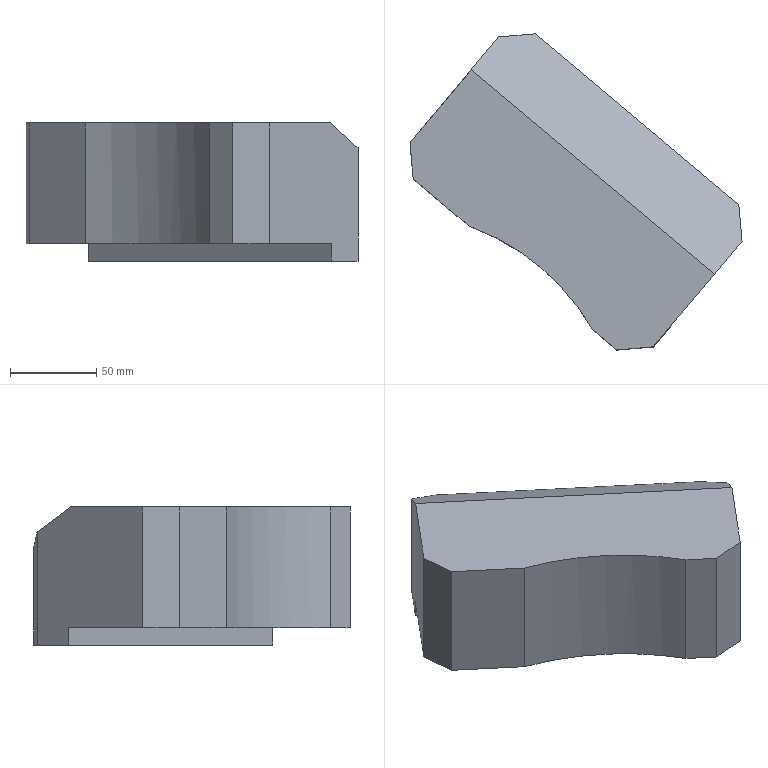Part | NX | features solid 2 | 1 solid | 31 faces | box 192.375 x 183.254 x 80 mm | volume 1311532 mm3 | plane 14 | cylinder 8 | cone 8 | spline 1 | commonest cylinder face diameters 10 x4 12 x4
STEP:
#1=CARTESIAN_POINT('',(626.964,495.071,0.000000024));
#2=VERTEX_POINT('',#1);
#3=CARTESIAN_POINT('',(621.964,495.071,0.000000024));
#4=DIRECTION('',(0.,0.,1.));
#5=DIRECTION('',(1.,0.,0.));
#6=AXIS2_PLACEMENT_3D('',#3,#4,#5);
#7=CIRCLE('',#6,5.);
#8=EDGE_CURVE('',#2,#2,#7,.T.);
#9=ORIENTED_EDGE('',*,*,#8,.T.);
#10=EDGE_LOOP('',(#9));
#11=FACE_BOUND('',#10,.T.);
#12=CARTESIAN_POINT('',(603.499,560.45,0.000000024));
#13=VERTEX_POINT('',#12);
#14=CARTESIAN_POINT('',(598.499,560.45,0.000000024));
#15=DIRECTION('',(0.,0.,1.));
#16=DIRECTION('',(1.,0.,0.));
#17=AXIS2_PLACEMENT_3D('',#14,#15,#16);
#18=CIRCLE('',#17,5.);
#19=EDGE_CURVE('',#13,#13,#18,.T.);
#20=ORIENTED_EDGE('',*,*,#19,.T.);
#21=EDGE_LOOP('',(#20));
#22=FACE_BOUND('',#21,.T.);
#23=CARTESIAN_POINT('',(650.461,521.883,0.000000024));
#24=VERTEX_POINT('',#23);
#25=CARTESIAN_POINT('',(644.461,521.883,0.000000024));
#26=DIRECTION('',(0.,0.,1.));
#27=DIRECTION('',(1.,0.,0.));
#28=AXIS2_PLACEMENT_3D('',#25,#26,#27);
#29=CIRCLE('',#28,6.);
#30=EDGE_CURVE('',#24,#24,#29,.T.);
#31=ORIENTED_EDGE('',*,*,#30,.T.);
#32=EDGE_LOOP('',(#31));
#33=FACE_BOUND('',#32,.T.);
#34=CARTESIAN_POINT('',(623.65,544.38,0.000000024));
#35=VERTEX_POINT('',#34);
#36=CARTESIAN_POINT('',(617.65,544.38,0.000000024));
#37=DIRECTION('',(0.,0.,1.));
#38=DIRECTION('',(1.,0.,0.));
#39=AXIS2_PLACEMENT_3D('',#36,#37,#38);
#40=CIRCLE('',#39,6.);
#41=EDGE_CURVE('',#35,#35,#40,.T.);
#42=ORIENTED_EDGE('',*,*,#41,.T.);
#43=EDGE_LOOP('',(#42));
#44=FACE_BOUND('',#43,.T.);
#45=CARTESIAN_POINT('',(523.703,550.108,0.000000024));
#46=VERTEX_POINT('',#45);
#47=CARTESIAN_POINT('',(595.572,489.803,0.000000024));
#48=VERTEX_POINT('',#47);
#49=CARTESIAN_POINT('',(523.703,550.108,0.000000024));
#50=CARTESIAN_POINT('',(531.205,547.402,0.000000024));
#51=CARTESIAN_POINT('',(545.792,540.631,0.000000024));
#52=CARTESIAN_POINT('',(565.448,526.903,0.000000024));
#53=CARTESIAN_POINT('',(582.431,509.864,0.000000024));
#54=CARTESIAN_POINT('',(591.599,496.685,0.000000024));
#55=CARTESIAN_POINT('',(595.572,489.803,0.000000024));
#56=B_SPLINE_CURVE_WITH_KNOTS('',3,(#49,#50,#51,#52,#53,#54,#55),.UNSPECIFIED.,.F.,.F.,(4,1,1,1,4),(0.2128,0.2368,0.2608,0.2847,0.3087),.UNSPECIFIED.);
#57=EDGE_CURVE('',#46,#48,#56,.T.);
#58=ORIENTED_EDGE('',*,*,#57,.F.);
#59=CARTESIAN_POINT('',(491.261,577.331,0.000000024));
#60=VERTEX_POINT('',#59);
#61=CARTESIAN_POINT('',(467.513,597.257,0.000000024));
#62=DIRECTION('',(0.766,-0.6428,0.));
#63=VECTOR('',#62,1000.);
#64=LINE('',#61,#63);
#65=EDGE_CURVE('',#60,#46,#64,.T.);
#66=ORIENTED_EDGE('',*,*,#65,.F.);
#67=CARTESIAN_POINT('',(489.412,598.463,0.000000024));
#68=VERTEX_POINT('',#67);
#69=CARTESIAN_POINT('',(491.261,577.331,0.000000024));
#70=DIRECTION('',(0.08716,-0.9962,0.));
#71=VECTOR('',#70,1000.);
#72=LINE('',#69,#71);
#73=EDGE_CURVE('',#68,#60,#72,.T.);
#74=ORIENTED_EDGE('',*,*,#73,.F.);
#75=CARTESIAN_POINT('',(525.408,641.362,0.000000024));
#76=VERTEX_POINT('',#75);
#77=CARTESIAN_POINT('',(527.979,644.426,0.000000024));
#78=DIRECTION('',(0.6428,0.766,0.));
#79=VECTOR('',#78,1000.);
#80=LINE('',#77,#79);
#81=EDGE_CURVE('',#76,#68,#80,.F.);
#82=ORIENTED_EDGE('',*,*,#81,.F.);
#83=CARTESIAN_POINT('',(666.36,523.089,0.000000024));
#84=VERTEX_POINT('',#83);
#85=CARTESIAN_POINT('',(513.151,651.646,0.000000024));
#86=DIRECTION('',(-0.766,0.6428,0.));
#87=VECTOR('',#86,1000.);
#88=LINE('',#85,#87);
#89=EDGE_CURVE('',#84,#76,#88,.T.);
#90=ORIENTED_EDGE('',*,*,#89,.F.);
#91=CARTESIAN_POINT('',(630.364,480.19,0.000000024));
#92=VERTEX_POINT('',#91);
#93=CARTESIAN_POINT('',(668.931,526.153,0.000000024));
#94=DIRECTION('',(0.6428,0.766,0.));
#95=VECTOR('',#94,1000.);
#96=LINE('',#93,#95);
#97=EDGE_CURVE('',#84,#92,#96,.F.);
#98=ORIENTED_EDGE('',*,*,#97,.T.);
#99=CARTESIAN_POINT('',(609.231,478.341,0.000000024));
#100=VERTEX_POINT('',#99);
#101=CARTESIAN_POINT('',(630.364,480.19,0.000000024));
#102=DIRECTION('',(-0.9962,-0.08716,0.));
#103=VECTOR('',#102,1000.);
#104=LINE('',#101,#103);
#105=EDGE_CURVE('',#100,#92,#104,.F.);
#106=ORIENTED_EDGE('',*,*,#105,.F.);
#107=CARTESIAN_POINT('',(467.513,597.257,0.000000024));
#108=DIRECTION('',(0.766,-0.6428,0.));
#109=VECTOR('',#108,1000.);
#110=LINE('',#107,#109);
#111=EDGE_CURVE('',#48,#100,#110,.T.);
#112=ORIENTED_EDGE('',*,*,#111,.F.);
#113=EDGE_LOOP('',(#58,#66,#74,#82,#90,#98,#106,#112));
#114=FACE_BOUND('',#113,.T.);
#115=CARTESIAN_POINT('',(510.525,592.775,0.000000024));
#116=VERTEX_POINT('',#115);
#117=CARTESIAN_POINT('',(505.525,592.775,0.000000024));
#118=DIRECTION('',(0.,0.,1.));
#119=DIRECTION('',(1.,0.,0.));
#120=AXIS2_PLACEMENT_3D('',#117,#118,#119);
#121=CIRCLE('',#120,5.);
#122=EDGE_CURVE('',#116,#116,#121,.T.);
#123=ORIENTED_EDGE('',*,*,#122,.T.);
#124=EDGE_LOOP('',(#123));
#125=FACE_BOUND('',#124,.T.);
#126=CARTESIAN_POINT('',(578.985,581.019,0.000000024));
#127=VERTEX_POINT('',#126);
#128=CARTESIAN_POINT('',(573.985,581.019,0.000000024));
#129=DIRECTION('',(0.,0.,1.));
#130=DIRECTION('',(1.,0.,0.));
#131=AXIS2_PLACEMENT_3D('',#128,#129,#130);
#132=CIRCLE('',#131,5.);
#133=EDGE_CURVE('',#127,#127,#132,.T.);
#134=ORIENTED_EDGE('',*,*,#133,.T.);
#135=EDGE_LOOP('',(#134));
#136=FACE_BOUND('',#135,.T.);
#137=CARTESIAN_POINT('',(560.834,597.089,0.000000024));
#138=VERTEX_POINT('',#137);
#139=CARTESIAN_POINT('',(554.834,597.089,0.000000024));
#140=DIRECTION('',(0.,0.,1.));
#141=DIRECTION('',(1.,0.,0.));
#142=AXIS2_PLACEMENT_3D('',#139,#140,#141);
#143=CIRCLE('',#142,6.);
#144=EDGE_CURVE('',#138,#138,#143,.T.);
#145=ORIENTED_EDGE('',*,*,#144,.T.);
#146=EDGE_LOOP('',(#145));
#147=FACE_BOUND('',#146,.T.);
#148=CARTESIAN_POINT('',(534.023,619.586,0.000000024));
#149=VERTEX_POINT('',#148);
#150=CARTESIAN_POINT('',(528.023,619.586,0.000000024));
#151=DIRECTION('',(0.,0.,1.));
#152=DIRECTION('',(1.,0.,0.));
#153=AXIS2_PLACEMENT_3D('',#150,#151,#152);
#154=CIRCLE('',#153,6.);
#155=EDGE_CURVE('',#149,#149,#154,.T.);
#156=ORIENTED_EDGE('',*,*,#155,.T.);
#157=EDGE_LOOP('',(#156));
#158=FACE_BOUND('',#157,.T.);
#159=CARTESIAN_POINT('',(515.722,654.71,0.000000024));
#160=DIRECTION('',(0.,0.,1.));
#161=DIRECTION('',(-1.,0.,0.));
#162=AXIS2_PLACEMENT_3D('',#159,#160,#161);
#163=PLANE('',#162);
#164=ADVANCED_FACE('',(#11,#22,#33,#44,#114,#125,#136,#147,#158),#163,.F.);
#165=CARTESIAN_POINT('',(595.572,489.803,70.));
#166=VERTEX_POINT('',#165);
#167=CARTESIAN_POINT('',(595.572,489.803,32.5));
#168=DIRECTION('',(0.,0.,1.));
#169=VECTOR('',#168,1000.);
#170=LINE('',#167,#169);
#171=EDGE_CURVE('',#166,#48,#170,.F.);
#172=ORIENTED_EDGE('',*,*,#171,.T.);
#173=ORIENTED_EDGE('',*,*,#111,.T.);
#174=CARTESIAN_POINT('',(609.231,478.341,70.));
#175=VERTEX_POINT('',#174);
#176=CARTESIAN_POINT('',(609.231,478.341,0.000000024));
#177=DIRECTION('',(0.,0.,-1.));
#178=VECTOR('',#177,1000.);
#179=LINE('',#176,#178);
#180=EDGE_CURVE('',#175,#100,#179,.T.);
#181=ORIENTED_EDGE('',*,*,#180,.F.);
#182=CARTESIAN_POINT('',(583.347,500.061,70.));
#183=DIRECTION('',(-0.766,0.6428,0.));
#184=VECTOR('',#183,1000.);
#185=LINE('',#182,#184);
#186=EDGE_CURVE('',#175,#166,#185,.T.);
#187=ORIENTED_EDGE('',*,*,#186,.T.);
#188=EDGE_LOOP('',(#172,#173,#181,#187));
#189=FACE_BOUND('',#188,.T.);
#190=CARTESIAN_POINT('',(467.513,597.257,0.000000024));
#191=DIRECTION('',(0.6428,0.766,0.));
#192=DIRECTION('',(0.766,-0.6428,0.));
#193=AXIS2_PLACEMENT_3D('',#190,#191,#192);
#194=PLANE('',#193);
#195=ADVANCED_FACE('',(#189),#194,.F.);
#196=CARTESIAN_POINT('',(523.703,550.108,70.));
#197=VERTEX_POINT('',#196);
#198=CARTESIAN_POINT('',(491.261,577.331,70.));
#199=VERTEX_POINT('',#198);
#200=CARTESIAN_POINT('',(583.347,500.061,70.));
#201=DIRECTION('',(-0.766,0.6428,0.));
#202=VECTOR('',#201,1000.);
#203=LINE('',#200,#202);
#204=EDGE_CURVE('',#197,#199,#203,.T.);
#205=ORIENTED_EDGE('',*,*,#204,.T.);
#206=CARTESIAN_POINT('',(491.261,577.331,0.000000024));
#207=DIRECTION('',(0.,0.,1.));
#208=VECTOR('',#207,1000.);
#209=LINE('',#206,#208);
#210=EDGE_CURVE('',#60,#199,#209,.T.);
#211=ORIENTED_EDGE('',*,*,#210,.F.);
#212=ORIENTED_EDGE('',*,*,#65,.T.);
#213=CARTESIAN_POINT('',(523.703,550.108,0.000000024));
#214=DIRECTION('',(0.,0.,1.));
#215=VECTOR('',#214,1000.);
#216=LINE('',#213,#215);
#217=EDGE_CURVE('',#46,#197,#216,.T.);
#218=ORIENTED_EDGE('',*,*,#217,.T.);
#219=EDGE_LOOP('',(#205,#211,#212,#218));
#220=FACE_BOUND('',#219,.T.);
#221=CARTESIAN_POINT('',(467.513,597.257,0.000000024));
#222=DIRECTION('',(0.6428,0.766,0.));
#223=DIRECTION('',(0.766,-0.6428,0.));
#224=AXIS2_PLACEMENT_3D('',#221,#222,#223);
#225=PLANE('',#224);
#226=ADVANCED_FACE('',(#220),#225,.F.);
#227=CARTESIAN_POINT('',(595.572,489.803,70.));
#228=CARTESIAN_POINT('',(591.553,496.763,70.));
#229=CARTESIAN_POINT('',(584.704,506.595,70.));
#230=CARTESIAN_POINT('',(573.845,518.482,70.));
#231=CARTESIAN_POINT('',(562.131,529.212,70.));
#232=CARTESIAN_POINT('',(549.111,538.318,70.));
#233=CARTESIAN_POINT('',(534.819,545.727,70.));
#234=CARTESIAN_POINT('',(527.454,548.755,70.));
#235=CARTESIAN_POINT('',(523.703,550.108,70.));
#236=B_SPLINE_CURVE_WITH_KNOTS('',3,(#227,#228,#229,#230,#231,#232,#233,#234,#235),.UNSPECIFIED.,.F.,.F.,(4,1,1,1,1,1,4),(0.02941,0.05349,0.06554,0.07758,0.1017,0.1137,0.1257),.UNSPECIFIED.);
#237=EDGE_CURVE('',#197,#166,#236,.F.);
#238=ORIENTED_EDGE('',*,*,#237,.T.);
#239=ORIENTED_EDGE('',*,*,#186,.F.);
#240=CARTESIAN_POINT('',(630.364,480.19,70.));
#241=VERTEX_POINT('',#240);
#242=CARTESIAN_POINT('',(630.364,480.19,70.));
#243=DIRECTION('',(0.9962,0.08716,0.));
#244=VECTOR('',#243,1000.);
#245=LINE('',#242,#244);
#246=EDGE_CURVE('',#241,#175,#245,.F.);
#247=ORIENTED_EDGE('',*,*,#246,.F.);
#248=CARTESIAN_POINT('',(665.717,522.323,70.));
#249=VERTEX_POINT('',#248);
#250=CARTESIAN_POINT('',(662.503,518.492,70.));
#251=DIRECTION('',(0.6428,0.766,0.));
#252=VECTOR('',#251,1000.);
#253=LINE('',#250,#252);
#254=EDGE_CURVE('',#249,#241,#253,.F.);
#255=ORIENTED_EDGE('',*,*,#254,.F.);
#256=CARTESIAN_POINT('',(524.765,640.596,70.));
#257=VERTEX_POINT('',#256);
#258=CARTESIAN_POINT('',(654.235,531.957,70.));
#259=DIRECTION('',(-0.766,0.6428,0.));
#260=VECTOR('',#259,1000.);
#261=LINE('',#258,#260);
#262=EDGE_CURVE('',#257,#249,#261,.F.);
#263=ORIENTED_EDGE('',*,*,#262,.F.);
#264=CARTESIAN_POINT('',(489.412,598.463,70.));
#265=VERTEX_POINT('',#264);
#266=CARTESIAN_POINT('',(527.979,644.426,70.));
#267=DIRECTION('',(0.6428,0.766,0.));
#268=VECTOR('',#267,1000.);
#269=LINE('',#266,#268);
#270=EDGE_CURVE('',#257,#265,#269,.F.);
#271=ORIENTED_EDGE('',*,*,#270,.T.);
#272=CARTESIAN_POINT('',(491.261,577.331,70.));
#273=DIRECTION('',(-0.08716,0.9962,0.));
#274=VECTOR('',#273,1000.);
#275=LINE('',#272,#274);
#276=EDGE_CURVE('',#199,#265,#275,.T.);
#277=ORIENTED_EDGE('',*,*,#276,.F.);
#278=ORIENTED_EDGE('',*,*,#204,.F.);
#279=EDGE_LOOP('',(#238,#239,#247,#255,#263,#271,#277,#278));
#280=FACE_BOUND('',#279,.T.);
#281=CARTESIAN_POINT('',(680.718,563.518,70.));
#282=DIRECTION('',(0.,0.,-1.));
#283=DIRECTION('',(-0.08716,0.9962,0.));
#284=AXIS2_PLACEMENT_3D('',#281,#282,#283);
#285=PLANE('',#284);
#286=ADVANCED_FACE('',(#280),#285,.F.);
#287=CARTESIAN_POINT('',(489.412,598.463,0.000000024));
#288=DIRECTION('',(0.,0.,1.));
#289=VECTOR('',#288,1000.);
#290=LINE('',#287,#289);
#291=EDGE_CURVE('',#265,#68,#290,.F.);
#292=ORIENTED_EDGE('',*,*,#291,.F.);
#293=ORIENTED_EDGE('',*,*,#270,.F.);
#294=CARTESIAN_POINT('',(540.835,659.747,55.566));
#295=VERTEX_POINT('',#294);
#296=CARTESIAN_POINT('',(528.609,645.177,66.547));
#297=DIRECTION('',(-0.5567,-0.6634,0.5));
#298=VECTOR('',#297,1000.);
#299=LINE('',#296,#298);
#300=EDGE_CURVE('',#295,#257,#299,.T.);
#301=ORIENTED_EDGE('',*,*,#300,.F.);
#302=CARTESIAN_POINT('',(540.835,659.747,-10.));
#303=VERTEX_POINT('',#302);
#304=CARTESIAN_POINT('',(540.835,659.747,0.000000024));
#305=DIRECTION('',(0.,0.,-1.));
#306=VECTOR('',#305,1000.);
#307=LINE('',#304,#306);
#308=EDGE_CURVE('',#303,#295,#307,.F.);
#309=ORIENTED_EDGE('',*,*,#308,.F.);
#310=CARTESIAN_POINT('',(525.408,641.362,-10.));
#311=VERTEX_POINT('',#310);
#312=CARTESIAN_POINT('',(550.477,671.237,-10.));
#313=DIRECTION('',(0.6428,0.766,0.));
#314=VECTOR('',#313,1000.);
#315=LINE('',#312,#314);
#316=EDGE_CURVE('',#303,#311,#315,.F.);
#317=ORIENTED_EDGE('',*,*,#316,.T.);
#318=CARTESIAN_POINT('',(525.408,641.362,0.000000024));
#319=DIRECTION('',(0.,0.,-1.));
#320=VECTOR('',#319,1000.);
#321=LINE('',#318,#320);
#322=EDGE_CURVE('',#311,#76,#321,.F.);
#323=ORIENTED_EDGE('',*,*,#322,.T.);
#324=ORIENTED_EDGE('',*,*,#81,.T.);
#325=EDGE_LOOP('',(#292,#293,#301,#309,#317,#323,#324));
#326=FACE_BOUND('',#325,.T.);
#327=CARTESIAN_POINT('',(527.979,644.426,0.000000024));
#328=DIRECTION('',(-0.766,0.6428,0.));
#329=DIRECTION('',(0.6428,0.766,0.));
#330=AXIS2_PLACEMENT_3D('',#327,#328,#329);
#331=PLANE('',#330);
#332=ADVANCED_FACE('',(#326),#331,.T.);
#333=CARTESIAN_POINT('',(681.787,541.474,55.566));
#334=VERTEX_POINT('',#333);
#335=CARTESIAN_POINT('',(660.996,516.696,74.24));
#336=DIRECTION('',(0.5567,0.6634,-0.5));
#337=VECTOR('',#336,1000.);
#338=LINE('',#335,#337);
#339=EDGE_CURVE('',#249,#334,#338,.T.);
#340=ORIENTED_EDGE('',*,*,#339,.F.);
#341=ORIENTED_EDGE('',*,*,#254,.T.);
#342=CARTESIAN_POINT('',(630.364,480.19,60.));
#343=DIRECTION('',(0.,0.,-1.));
#344=VECTOR('',#343,1000.);
#345=LINE('',#342,#344);
#346=EDGE_CURVE('',#92,#241,#345,.F.);
#347=ORIENTED_EDGE('',*,*,#346,.F.);
#348=ORIENTED_EDGE('',*,*,#97,.F.);
#349=CARTESIAN_POINT('',(666.36,523.089,-10.));
#350=VERTEX_POINT('',#349);
#351=CARTESIAN_POINT('',(666.36,523.089,0.000000024));
#352=DIRECTION('',(0.,0.,-1.));
#353=VECTOR('',#352,1000.);
#354=LINE('',#351,#353);
#355=EDGE_CURVE('',#350,#84,#354,.F.);
#356=ORIENTED_EDGE('',*,*,#355,.F.);
#357=CARTESIAN_POINT('',(681.787,541.474,-10.));
#358=VERTEX_POINT('',#357);
#359=CARTESIAN_POINT('',(691.429,552.964,-10.));
#360=DIRECTION('',(0.6428,0.766,0.));
#361=VECTOR('',#360,1000.);
#362=LINE('',#359,#361);
#363=EDGE_CURVE('',#358,#350,#362,.F.);
#364=ORIENTED_EDGE('',*,*,#363,.F.);
#365=CARTESIAN_POINT('',(681.787,541.474,-10.));
#366=DIRECTION('',(0.,0.,1.));
#367=VECTOR('',#366,1000.);
#368=LINE('',#365,#367);
#369=EDGE_CURVE('',#334,#358,#368,.F.);
#370=ORIENTED_EDGE('',*,*,#369,.F.);
#371=EDGE_LOOP('',(#340,#341,#347,#348,#356,#364,#370));
#372=FACE_BOUND('',#371,.T.);
#373=CARTESIAN_POINT('',(668.931,526.153,0.000000024));
#374=DIRECTION('',(-0.766,0.6428,0.));
#375=DIRECTION('',(0.6428,0.766,0.));
#376=AXIS2_PLACEMENT_3D('',#373,#374,#375);
#377=PLANE('',#376);
#378=ADVANCED_FACE('',(#372),#377,.F.);
#379=CARTESIAN_POINT('',(679.938,562.606,-10.));
#380=VERTEX_POINT('',#379);
#381=CARTESIAN_POINT('',(679.938,562.606,46.906));
#382=VERTEX_POINT('',#381);
#383=CARTESIAN_POINT('',(679.938,562.606,60.));
#384=DIRECTION('',(0.,0.,-1.));
#385=VECTOR('',#384,1000.);
#386=LINE('',#383,#385);
#387=EDGE_CURVE('',#380,#382,#386,.F.);
#388=ORIENTED_EDGE('',*,*,#387,.F.);
#389=CARTESIAN_POINT('',(561.967,661.596,-10.));
#390=VERTEX_POINT('',#389);
#391=CARTESIAN_POINT('',(668.447,572.248,-10.));
#392=DIRECTION('',(-0.766,0.6428,0.));
#393=VECTOR('',#392,1000.);
#394=LINE('',#391,#393);
#395=EDGE_CURVE('',#380,#390,#394,.T.);
#396=ORIENTED_EDGE('',*,*,#395,.T.);
#397=CARTESIAN_POINT('',(561.967,661.596,46.906));
#398=VERTEX_POINT('',#397);
#399=CARTESIAN_POINT('',(561.967,661.596,0.000000024));
#400=DIRECTION('',(0.,0.,1.));
#401=VECTOR('',#400,1000.);
#402=LINE('',#399,#401);
#403=EDGE_CURVE('',#398,#390,#402,.F.);
#404=ORIENTED_EDGE('',*,*,#403,.F.);
#405=CARTESIAN_POINT('',(679.946,562.599,46.906));
#406=DIRECTION('',(-0.766,0.6428,0.));
#407=VECTOR('',#406,1000.);
#408=LINE('',#405,#407);
#409=EDGE_CURVE('',#382,#398,#408,.T.);
#410=ORIENTED_EDGE('',*,*,#409,.F.);
#411=EDGE_LOOP('',(#388,#396,#404,#410));
#412=FACE_BOUND('',#411,.T.);
#413=CARTESIAN_POINT('',(706.75,540.109,0.000000024));
#414=DIRECTION('',(0.6428,0.766,0.));
#415=DIRECTION('',(0.766,-0.6428,0.));
#416=AXIS2_PLACEMENT_3D('',#413,#414,#415);
#417=PLANE('',#416);
#418=ADVANCED_FACE('',(#412),#417,.T.);
#419=ORIENTED_EDGE('',*,*,#395,.F.);
#420=CARTESIAN_POINT('',(679.938,562.606,-10.));
#421=DIRECTION('',(0.08716,-0.9962,0.));
#422=VECTOR('',#421,1000.);
#423=LINE('',#420,#422);
#424=EDGE_CURVE('',#358,#380,#423,.F.);
#425=ORIENTED_EDGE('',*,*,#424,.F.);
#426=ORIENTED_EDGE('',*,*,#363,.T.);
#427=CARTESIAN_POINT('',(643.379,542.372,-10.));
#428=DIRECTION('',(0.766,-0.6428,0.));
#429=VECTOR('',#428,1000.);
#430=LINE('',#427,#429);
#431=EDGE_CURVE('',#350,#311,#430,.F.);
#432=ORIENTED_EDGE('',*,*,#431,.T.);
#433=ORIENTED_EDGE('',*,*,#316,.F.);
#434=CARTESIAN_POINT('',(540.835,659.747,-10.));
#435=DIRECTION('',(-0.9962,-0.08716,0.));
#436=VECTOR('',#435,1000.);
#437=LINE('',#434,#436);
#438=EDGE_CURVE('',#390,#303,#437,.T.);
#439=ORIENTED_EDGE('',*,*,#438,.F.);
#440=EDGE_LOOP('',(#419,#425,#426,#432,#433,#439));
#441=FACE_BOUND('',#440,.T.);
#442=CARTESIAN_POINT('',(668.447,572.248,-10.));
#443=DIRECTION('',(0.,0.,-1.));
#444=DIRECTION('',(-0.766,0.6428,0.));
#445=AXIS2_PLACEMENT_3D('',#442,#443,#444);
#446=PLANE('',#445);
#447=ADVANCED_FACE('',(#441),#446,.T.);
#448=ORIENTED_EDGE('',*,*,#89,.T.);
#449=ORIENTED_EDGE('',*,*,#322,.F.);
#450=ORIENTED_EDGE('',*,*,#431,.F.);
#451=ORIENTED_EDGE('',*,*,#355,.T.);
#452=EDGE_LOOP('',(#448,#449,#450,#451));
#453=FACE_BOUND('',#452,.T.);
#454=CARTESIAN_POINT('',(643.379,542.372,-10.));
#455=DIRECTION('',(-0.6428,-0.766,0.));
#456=DIRECTION('',(-0.766,0.6428,0.));
#457=AXIS2_PLACEMENT_3D('',#454,#455,#456);
#458=PLANE('',#457);
#459=ADVANCED_FACE('',(#453),#458,.T.);
#460=ORIENTED_EDGE('',*,*,#403,.T.);
#461=ORIENTED_EDGE('',*,*,#438,.T.);
#462=ORIENTED_EDGE('',*,*,#308,.T.);
#463=CARTESIAN_POINT('',(560.205,661.441,47.628));
#464=DIRECTION('',(-0.9223,-0.08069,0.378));
#465=VECTOR('',#464,1000.);
#466=LINE('',#463,#465);
#467=EDGE_CURVE('',#398,#295,#466,.T.);
#468=ORIENTED_EDGE('',*,*,#467,.F.);
#469=EDGE_LOOP('',(#460,#461,#462,#468));
#470=FACE_BOUND('',#469,.T.);
#471=CARTESIAN_POINT('',(540.835,659.747,0.000000024));
#472=DIRECTION('',(0.08716,-0.9962,0.));
#473=DIRECTION('',(-0.9962,-0.08716,0.));
#474=AXIS2_PLACEMENT_3D('',#471,#472,#473);
#475=PLANE('',#474);
#476=ADVANCED_FACE('',(#470),#475,.F.);
#477=ORIENTED_EDGE('',*,*,#369,.T.);
#478=ORIENTED_EDGE('',*,*,#424,.T.);
#479=ORIENTED_EDGE('',*,*,#387,.T.);
#480=CARTESIAN_POINT('',(678.508,578.957,40.205));
#481=DIRECTION('',(0.08069,-0.9223,0.378));
#482=VECTOR('',#481,1000.);
#483=LINE('',#480,#482);
#484=EDGE_CURVE('',#334,#382,#483,.F.);
#485=ORIENTED_EDGE('',*,*,#484,.F.);
#486=EDGE_LOOP('',(#477,#478,#479,#485));
#487=FACE_BOUND('',#486,.T.);
#488=CARTESIAN_POINT('',(679.938,562.606,0.000000024));
#489=DIRECTION('',(0.9962,0.08716,0.));
#490=DIRECTION('',(0.08716,-0.9962,0.));
#491=AXIS2_PLACEMENT_3D('',#488,#489,#490);
#492=PLANE('',#491);
#493=ADVANCED_FACE('',(#487),#492,.T.);
#494=ORIENTED_EDGE('',*,*,#105,.T.);
#495=ORIENTED_EDGE('',*,*,#346,.T.);
#496=ORIENTED_EDGE('',*,*,#246,.T.);
#497=ORIENTED_EDGE('',*,*,#180,.T.);
#498=EDGE_LOOP('',(#494,#495,#496,#497));
#499=FACE_BOUND('',#498,.T.);
#500=CARTESIAN_POINT('',(630.364,480.19,0.000000024));
#501=DIRECTION('',(-0.08716,0.9962,0.));
#502=DIRECTION('',(0.9962,0.08716,0.));
#503=AXIS2_PLACEMENT_3D('',#500,#501,#502);
#504=PLANE('',#503);
#505=ADVANCED_FACE('',(#499),#504,.F.);
#506=ORIENTED_EDGE('',*,*,#73,.T.);
#507=ORIENTED_EDGE('',*,*,#210,.T.);
#508=ORIENTED_EDGE('',*,*,#276,.T.);
#509=ORIENTED_EDGE('',*,*,#291,.T.);
#510=EDGE_LOOP('',(#506,#507,#508,#509));
#511=FACE_BOUND('',#510,.T.);
#512=CARTESIAN_POINT('',(491.261,577.331,0.000000024));
#513=DIRECTION('',(-0.9962,-0.08716,0.));
#514=DIRECTION('',(-0.08716,0.9962,0.));
#515=AXIS2_PLACEMENT_3D('',#512,#513,#514);
#516=PLANE('',#515);
#517=ADVANCED_FACE('',(#511),#516,.T.);
#518=ORIENTED_EDGE('',*,*,#467,.T.);
#519=ORIENTED_EDGE('',*,*,#300,.T.);
#520=ORIENTED_EDGE('',*,*,#262,.T.);
#521=ORIENTED_EDGE('',*,*,#339,.T.);
#522=ORIENTED_EDGE('',*,*,#484,.T.);
#523=ORIENTED_EDGE('',*,*,#409,.T.);
#524=EDGE_LOOP('',(#518,#519,#520,#521,#522,#523));
#525=FACE_BOUND('',#524,.T.);
#526=CARTESIAN_POINT('',(658.079,536.539,66.547));
#527=DIRECTION('',(-0.3214,-0.383,-0.866));
#528=DIRECTION('',(0.8968,0.1706,-0.4082));
#529=AXIS2_PLACEMENT_3D('',#526,#527,#528);
#530=PLANE('',#529);
#531=ADVANCED_FACE('',(#525),#530,.F.);
#532=ORIENTED_EDGE('',*,*,#217,.F.);
#533=ORIENTED_EDGE('',*,*,#57,.T.);
#534=ORIENTED_EDGE('',*,*,#171,.F.);
#535=ORIENTED_EDGE('',*,*,#237,.F.);
#536=EDGE_LOOP('',(#532,#533,#534,#535));
#537=FACE_BOUND('',#536,.T.);
#538=CARTESIAN_POINT('',(523.703,550.108,0.000000024));
#539=CARTESIAN_POINT('',(523.703,550.108,70.));
#540=CARTESIAN_POINT('',(531.233,547.392,0.000000024));
#541=CARTESIAN_POINT('',(531.233,547.392,70.));
#542=CARTESIAN_POINT('',(542.036,542.382,0.000000024));
#543=CARTESIAN_POINT('',(542.036,542.382,70.));
#544=CARTESIAN_POINT('',(555.597,533.785,0.000000024));
#545=CARTESIAN_POINT('',(555.597,533.785,70.));
#546=CARTESIAN_POINT('',(568.47,523.908,0.000000024));
#547=CARTESIAN_POINT('',(568.47,523.908,70.));
#548=CARTESIAN_POINT('',(582.535,509.722,0.000000024));
#549=CARTESIAN_POINT('',(582.535,509.722,70.));
#550=CARTESIAN_POINT('',(591.647,496.601,0.000000024));
#551=CARTESIAN_POINT('',(591.647,496.601,70.));
#552=CARTESIAN_POINT('',(595.572,489.803,0.000000024));
#553=CARTESIAN_POINT('',(595.572,489.803,70.));
#554=B_SPLINE_SURFACE_WITH_KNOTS('',3,1,((#538,#539),(#540,#541),(#542,#543),(#544,#545),(#546,#547),(#548,#549),(#550,#551),(#552,#553)),.SURF_OF_LINEAR_EXTRUSION.,.F.,.F.,.F.,(4,1,1,1,1,4),(2,2),(0.06717,0.283,0.391,0.4989,0.7148,0.9307),(0.,1.),.UNSPECIFIED.);
#555=ADVANCED_FACE('',(#537),#554,.T.);
#556=ORIENTED_EDGE('',*,*,#122,.F.);
#557=EDGE_LOOP('',(#556));
#558=FACE_BOUND('',#557,.T.);
#559=CARTESIAN_POINT('',(510.525,592.775,30.));
#560=VERTEX_POINT('',#559);
#561=CARTESIAN_POINT('',(505.525,592.775,30.));
#562=DIRECTION('',(0.,0.,1.));
#563=DIRECTION('',(1.,0.,0.));
#564=AXIS2_PLACEMENT_3D('',#561,#562,#563);
#565=CIRCLE('',#564,5.);
#566=EDGE_CURVE('',#560,#560,#565,.T.);
#567=ORIENTED_EDGE('',*,*,#566,.T.);
#568=EDGE_LOOP('',(#567));
#569=FACE_BOUND('',#568,.T.);
#570=CARTESIAN_POINT('',(505.525,592.775,0.000000024));
#571=DIRECTION('',(0.,0.,1.));
#572=DIRECTION('',(1.,0.,0.));
#573=AXIS2_PLACEMENT_3D('',#570,#571,#572);
#574=CYLINDRICAL_SURFACE('',#573,5.);
#575=ADVANCED_FACE('',(#558,#569),#574,.F.);
#576=ORIENTED_EDGE('',*,*,#133,.F.);
#577=EDGE_LOOP('',(#576));
#578=FACE_BOUND('',#577,.T.);
#579=CARTESIAN_POINT('',(578.985,581.019,30.));
#580=VERTEX_POINT('',#579);
#581=CARTESIAN_POINT('',(573.985,581.019,30.));
#582=DIRECTION('',(0.,0.,1.));
#583=DIRECTION('',(1.,0.,0.));
#584=AXIS2_PLACEMENT_3D('',#581,#582,#583);
#585=CIRCLE('',#584,5.);
#586=EDGE_CURVE('',#580,#580,#585,.T.);
#587=ORIENTED_EDGE('',*,*,#586,.T.);
#588=EDGE_LOOP('',(#587));
#589=FACE_BOUND('',#588,.T.);
#590=CARTESIAN_POINT('',(573.985,581.019,0.000000024));
#591=DIRECTION('',(0.,0.,1.));
#592=DIRECTION('',(1.,0.,0.));
#593=AXIS2_PLACEMENT_3D('',#590,#591,#592);
#594=CYLINDRICAL_SURFACE('',#593,5.);
#595=ADVANCED_FACE('',(#578,#589),#594,.F.);
#596=CARTESIAN_POINT('',(560.834,597.089,35.));
#597=VERTEX_POINT('',#596);
#598=CARTESIAN_POINT('',(554.834,597.089,35.));
#599=DIRECTION('',(0.,0.,1.));
#600=DIRECTION('',(1.,0.,0.));
#601=AXIS2_PLACEMENT_3D('',#598,#599,#600);
#602=CIRCLE('',#601,6.);
#603=EDGE_CURVE('',#597,#597,#602,.T.);
#604=ORIENTED_EDGE('',*,*,#603,.F.);
#605=EDGE_LOOP('',(#604));
#606=FACE_BOUND('',#605,.T.);
#607=CARTESIAN_POINT('',(554.834,597.089,38.605));
#608=VERTEX_POINT('',#607);
#609=VERTEX_LOOP('',#608);
#610=FACE_BOUND('',#609,.T.);
#611=CARTESIAN_POINT('',(554.834,597.089,35.));
#612=DIRECTION('',(0.,0.,-1.));
#613=DIRECTION('',(-1.,0.,0.));
#614=AXIS2_PLACEMENT_3D('',#611,#612,#613);
#615=CONICAL_SURFACE('',#614,6.,1.03);
#616=ADVANCED_FACE('',(#606,#610),#615,.F.);
#617=ORIENTED_EDGE('',*,*,#603,.T.);
#618=EDGE_LOOP('',(#617));
#619=FACE_BOUND('',#618,.T.);
#620=ORIENTED_EDGE('',*,*,#144,.F.);
#621=EDGE_LOOP('',(#620));
#622=FACE_BOUND('',#621,.T.);
#623=CARTESIAN_POINT('',(554.834,597.089,0.000000024));
#624=DIRECTION('',(0.,0.,1.));
#625=DIRECTION('',(1.,0.,0.));
#626=AXIS2_PLACEMENT_3D('',#623,#624,#625);
#627=CYLINDRICAL_SURFACE('',#626,6.);
#628=ADVANCED_FACE('',(#619,#622),#627,.F.);
#629=CARTESIAN_POINT('',(534.023,619.586,35.));
#630=VERTEX_POINT('',#629);
#631=CARTESIAN_POINT('',(528.023,619.586,35.));
#632=DIRECTION('',(0.,0.,1.));
#633=DIRECTION('',(1.,0.,0.));
#634=AXIS2_PLACEMENT_3D('',#631,#632,#633);
#635=CIRCLE('',#634,6.);
#636=EDGE_CURVE('',#630,#630,#635,.T.);
#637=ORIENTED_EDGE('',*,*,#636,.F.);
#638=EDGE_LOOP('',(#637));
#639=FACE_BOUND('',#638,.T.);
#640=CARTESIAN_POINT('',(528.023,619.586,38.605));
#641=VERTEX_POINT('',#640);
#642=VERTEX_LOOP('',#641);
#643=FACE_BOUND('',#642,.T.);
#644=CARTESIAN_POINT('',(528.023,619.586,35.));
#645=DIRECTION('',(0.,0.,-1.));
#646=DIRECTION('',(-1.,0.,0.));
#647=AXIS2_PLACEMENT_3D('',#644,#645,#646);
#648=CONICAL_SURFACE('',#647,6.,1.03);
#649=ADVANCED_FACE('',(#639,#643),#648,.F.);
#650=ORIENTED_EDGE('',*,*,#636,.T.);
#651=EDGE_LOOP('',(#650));
#652=FACE_BOUND('',#651,.T.);
#653=ORIENTED_EDGE('',*,*,#155,.F.);
#654=EDGE_LOOP('',(#653));
#655=FACE_BOUND('',#654,.T.);
#656=CARTESIAN_POINT('',(528.023,619.586,0.000000024));
#657=DIRECTION('',(0.,0.,1.));
#658=DIRECTION('',(1.,0.,0.));
#659=AXIS2_PLACEMENT_3D('',#656,#657,#658);
#660=CYLINDRICAL_SURFACE('',#659,6.);
#661=ADVANCED_FACE('',(#652,#655),#660,.F.);
#662=CARTESIAN_POINT('',(623.65,544.38,35.));
#663=VERTEX_POINT('',#662);
#664=CARTESIAN_POINT('',(617.65,544.38,35.));
#665=DIRECTION('',(0.,0.,1.));
#666=DIRECTION('',(1.,0.,0.));
#667=AXIS2_PLACEMENT_3D('',#664,#665,#666);
#668=CIRCLE('',#667,6.);
#669=EDGE_CURVE('',#663,#663,#668,.T.);
#670=ORIENTED_EDGE('',*,*,#669,.F.);
#671=EDGE_LOOP('',(#670));
#672=FACE_BOUND('',#671,.T.);
#673=CARTESIAN_POINT('',(617.65,544.38,38.605));
#674=VERTEX_POINT('',#673);
#675=VERTEX_LOOP('',#674);
#676=FACE_BOUND('',#675,.T.);
#677=CARTESIAN_POINT('',(617.65,544.38,35.));
#678=DIRECTION('',(0.,0.,-1.));
#679=DIRECTION('',(-1.,0.,0.));
#680=AXIS2_PLACEMENT_3D('',#677,#678,#679);
#681=CONICAL_SURFACE('',#680,6.,1.03);
#682=ADVANCED_FACE('',(#672,#676),#681,.F.);
#683=ORIENTED_EDGE('',*,*,#669,.T.);
#684=EDGE_LOOP('',(#683));
#685=FACE_BOUND('',#684,.T.);
#686=ORIENTED_EDGE('',*,*,#41,.F.);
#687=EDGE_LOOP('',(#686));
#688=FACE_BOUND('',#687,.T.);
#689=CARTESIAN_POINT('',(617.65,544.38,0.000000024));
#690=DIRECTION('',(0.,0.,1.));
#691=DIRECTION('',(1.,0.,0.));
#692=AXIS2_PLACEMENT_3D('',#689,#690,#691);
#693=CYLINDRICAL_SURFACE('',#692,6.);
#694=ADVANCED_FACE('',(#685,#688),#693,.F.);
#695=CARTESIAN_POINT('',(650.461,521.883,35.));
#696=VERTEX_POINT('',#695);
#697=CARTESIAN_POINT('',(644.461,521.883,35.));
#698=DIRECTION('',(0.,0.,1.));
#699=DIRECTION('',(1.,0.,0.));
#700=AXIS2_PLACEMENT_3D('',#697,#698,#699);
#701=CIRCLE('',#700,6.);
#702=EDGE_CURVE('',#696,#696,#701,.T.);
#703=ORIENTED_EDGE('',*,*,#702,.F.);
#704=EDGE_LOOP('',(#703));
#705=FACE_BOUND('',#704,.T.);
#706=CARTESIAN_POINT('',(644.461,521.883,38.605));
#707=VERTEX_POINT('',#706);
#708=VERTEX_LOOP('',#707);
#709=FACE_BOUND('',#708,.T.);
#710=CARTESIAN_POINT('',(644.461,521.883,35.));
#711=DIRECTION('',(0.,0.,-1.));
#712=DIRECTION('',(-1.,0.,0.));
#713=AXIS2_PLACEMENT_3D('',#710,#711,#712);
#714=CONICAL_SURFACE('',#713,6.,1.03);
#715=ADVANCED_FACE('',(#705,#709),#714,.F.);
#716=ORIENTED_EDGE('',*,*,#702,.T.);
#717=EDGE_LOOP('',(#716));
#718=FACE_BOUND('',#717,.T.);
#719=ORIENTED_EDGE('',*,*,#30,.F.);
#720=EDGE_LOOP('',(#719));
#721=FACE_BOUND('',#720,.T.);
#722=CARTESIAN_POINT('',(644.461,521.883,0.000000024));
#723=DIRECTION('',(0.,0.,1.));
#724=DIRECTION('',(1.,0.,0.));
#725=AXIS2_PLACEMENT_3D('',#722,#723,#724);
#726=CYLINDRICAL_SURFACE('',#725,6.);
#727=ADVANCED_FACE('',(#718,#721),#726,.F.);
#728=ORIENTED_EDGE('',*,*,#19,.F.);
#729=EDGE_LOOP('',(#728));
#730=FACE_BOUND('',#729,.T.);
#731=CARTESIAN_POINT('',(603.499,560.45,30.));
#732=VERTEX_POINT('',#731);
#733=CARTESIAN_POINT('',(598.499,560.45,30.));
#734=DIRECTION('',(0.,0.,1.));
#735=DIRECTION('',(1.,0.,0.));
#736=AXIS2_PLACEMENT_3D('',#733,#734,#735);
#737=CIRCLE('',#736,5.);
#738=EDGE_CURVE('',#732,#732,#737,.T.);
#739=ORIENTED_EDGE('',*,*,#738,.T.);
#740=EDGE_LOOP('',(#739));
#741=FACE_BOUND('',#740,.T.);
#742=CARTESIAN_POINT('',(598.499,560.45,0.000000024));
#743=DIRECTION('',(0.,0.,1.));
#744=DIRECTION('',(1.,0.,0.));
#745=AXIS2_PLACEMENT_3D('',#742,#743,#744);
#746=CYLINDRICAL_SURFACE('',#745,5.);
#747=ADVANCED_FACE('',(#730,#741),#746,.F.);
#748=ORIENTED_EDGE('',*,*,#8,.F.);
#749=EDGE_LOOP('',(#748));
#750=FACE_BOUND('',#749,.T.);
#751=CARTESIAN_POINT('',(626.964,495.071,30.));
#752=VERTEX_POINT('',#751);
#753=CARTESIAN_POINT('',(621.964,495.071,30.));
#754=DIRECTION('',(0.,0.,1.));
#755=DIRECTION('',(1.,0.,0.));
#756=AXIS2_PLACEMENT_3D('',#753,#754,#755);
#757=CIRCLE('',#756,5.);
#758=EDGE_CURVE('',#752,#752,#757,.T.);
#759=ORIENTED_EDGE('',*,*,#758,.T.);
#760=EDGE_LOOP('',(#759));
#761=FACE_BOUND('',#760,.T.);
#762=CARTESIAN_POINT('',(621.964,495.071,0.000000024));
#763=DIRECTION('',(0.,0.,1.));
#764=DIRECTION('',(1.,0.,0.));
#765=AXIS2_PLACEMENT_3D('',#762,#763,#764);
#766=CYLINDRICAL_SURFACE('',#765,5.);
#767=ADVANCED_FACE('',(#750,#761),#766,.F.);
#768=ORIENTED_EDGE('',*,*,#566,.F.);
#769=EDGE_LOOP('',(#768));
#770=FACE_BOUND('',#769,.T.);
#771=CARTESIAN_POINT('',(505.525,592.775,33.004));
#772=VERTEX_POINT('',#771);
#773=VERTEX_LOOP('',#772);
#774=FACE_BOUND('',#773,.T.);
#775=CARTESIAN_POINT('',(505.525,592.775,30.));
#776=DIRECTION('',(0.,0.,-1.));
#777=DIRECTION('',(-1.,0.,0.));
#778=AXIS2_PLACEMENT_3D('',#775,#776,#777);
#779=CONICAL_SURFACE('',#778,5.,1.03);
#780=ADVANCED_FACE('',(#770,#774),#779,.F.);
#781=ORIENTED_EDGE('',*,*,#586,.F.);
#782=EDGE_LOOP('',(#781));
#783=FACE_BOUND('',#782,.T.);
#784=CARTESIAN_POINT('',(573.985,581.019,33.004));
#785=VERTEX_POINT('',#784);
#786=VERTEX_LOOP('',#785);
#787=FACE_BOUND('',#786,.T.);
#788=CARTESIAN_POINT('',(573.985,581.019,30.));
#789=DIRECTION('',(0.,0.,-1.));
#790=DIRECTION('',(-1.,0.,0.));
#791=AXIS2_PLACEMENT_3D('',#788,#789,#790);
#792=CONICAL_SURFACE('',#791,5.,1.03);
#793=ADVANCED_FACE('',(#783,#787),#792,.F.);
#794=ORIENTED_EDGE('',*,*,#738,.F.);
#795=EDGE_LOOP('',(#794));
#796=FACE_BOUND('',#795,.T.);
#797=CARTESIAN_POINT('',(598.499,560.45,33.004));
#798=VERTEX_POINT('',#797);
#799=VERTEX_LOOP('',#798);
#800=FACE_BOUND('',#799,.T.);
#801=CARTESIAN_POINT('',(598.499,560.45,30.));
#802=DIRECTION('',(0.,0.,-1.));
#803=DIRECTION('',(-1.,0.,0.));
#804=AXIS2_PLACEMENT_3D('',#801,#802,#803);
#805=CONICAL_SURFACE('',#804,5.,1.03);
#806=ADVANCED_FACE('',(#796,#800),#805,.F.);
#807=ORIENTED_EDGE('',*,*,#758,.F.);
#808=EDGE_LOOP('',(#807));
#809=FACE_BOUND('',#808,.T.);
#810=CARTESIAN_POINT('',(621.964,495.071,33.004));
#811=VERTEX_POINT('',#810);
#812=VERTEX_LOOP('',#811);
#813=FACE_BOUND('',#812,.T.);
#814=CARTESIAN_POINT('',(621.964,495.071,30.));
#815=DIRECTION('',(0.,0.,-1.));
#816=DIRECTION('',(-1.,0.,0.));
#817=AXIS2_PLACEMENT_3D('',#814,#815,#816);
#818=CONICAL_SURFACE('',#817,5.,1.03);
#819=ADVANCED_FACE('',(#809,#813),#818,.F.);
#820=CLOSED_SHELL('',(#164,#195,#226,#286,#332,#378,#418,#447,#459,#476,#493,#505,#517,#531,#555,#575,#595,#616,#628,#649,#661,#682,#694,#715,#727,#747,#767,#780,#793,#806,#819));
#821=MANIFOLD_SOLID_BREP('',#820);
#822=(LENGTH_UNIT()NAMED_UNIT(*)SI_UNIT(.MILLI.,.METRE.));
#823=UNCERTAINTY_MEASURE_WITH_UNIT(LENGTH_MEASURE(0.0508),#822,'','');
#824=(NAMED_UNIT(*)PLANE_ANGLE_UNIT()SI_UNIT($,.RADIAN.));
#825=(NAMED_UNIT(*)SI_UNIT($,.STERADIAN.)SOLID_ANGLE_UNIT());
#826=(GEOMETRIC_REPRESENTATION_CONTEXT(3)GLOBAL_UNCERTAINTY_ASSIGNED_CONTEXT((#823))GLOBAL_UNIT_ASSIGNED_CONTEXT((#822,#824,#825))REPRESENTATION_CONTEXT('',''));
#827=ADVANCED_BREP_SHAPE_REPRESENTATION('',(#821),#826);